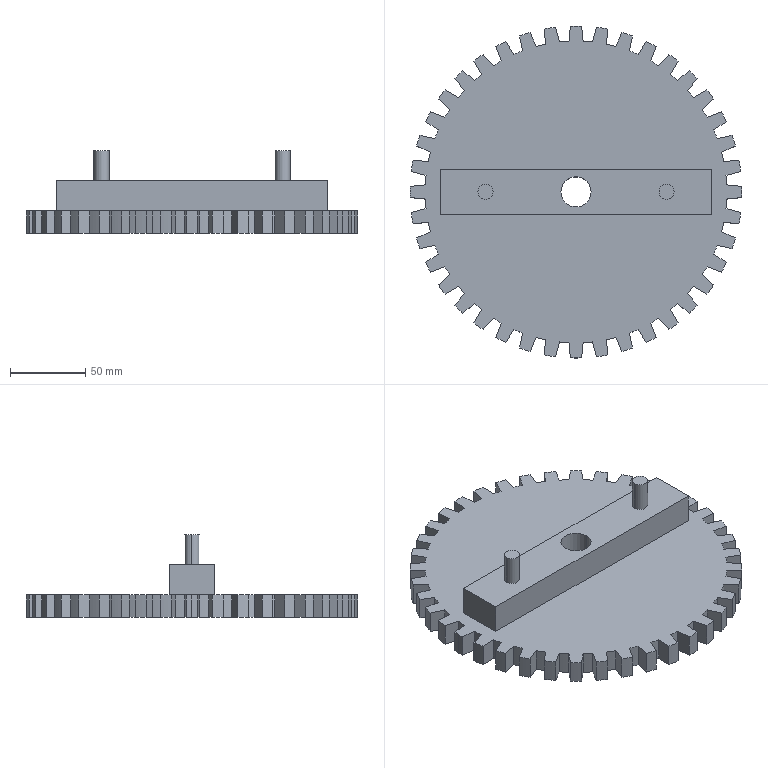Part | SolidWorks | features ICE 2, Extrusion 1 | 1 solid | 176 faces | box 220 x 220 x 55 mm | volume 621975 mm3 | plane 89 | cylinder 87 | commonest cylinder face diameters 220 x41 200 x40 10 x4 20 x2